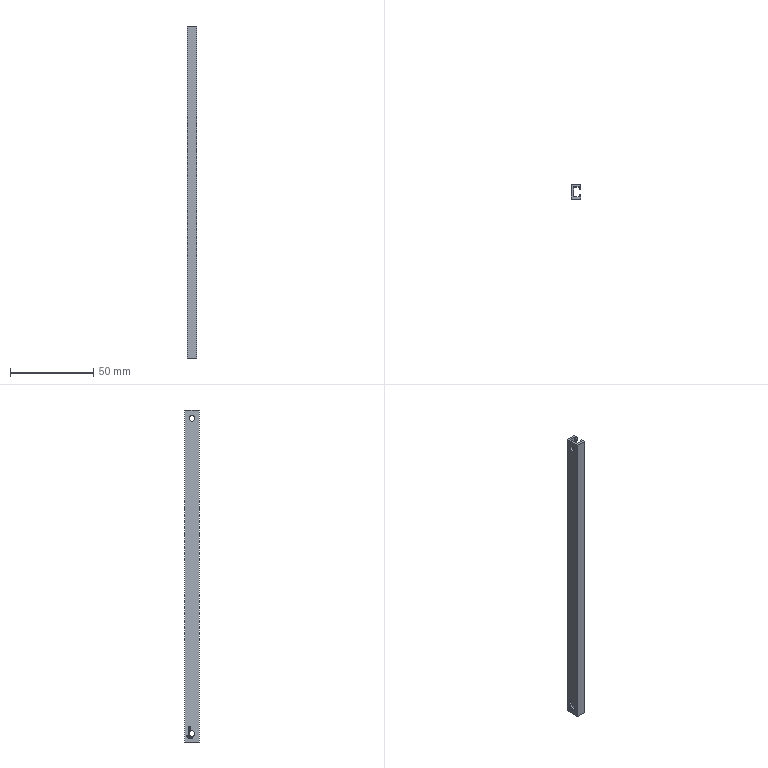Part | SolidWorks | features ICE 3, Extrusion 1 | 1 solid | 77 faces | box 6 x 9 x 200 mm | volume 5872 mm3 | plane 51 | spline 18 | cylinder 8 | commonest cylinder face diameters 3.5 x4 6 x4